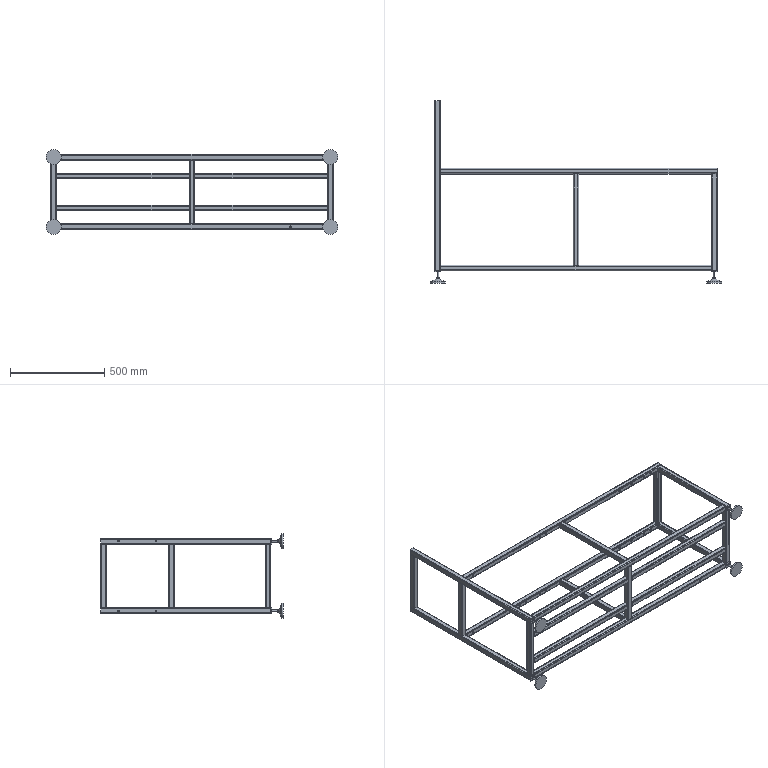Part | SolidWorks | features CompositeCurve 4, AEMSimFeature 1 | 36 solids | 716 faces | box 1550 x 971 x 450 mm | volume 4239958 mm3 | plane 304 | cylinder 276 | cone 136 | commonest cylinder face diameters 5.2 x80 10.4 x80 9 x44 7 x16 10 x16 8 x8